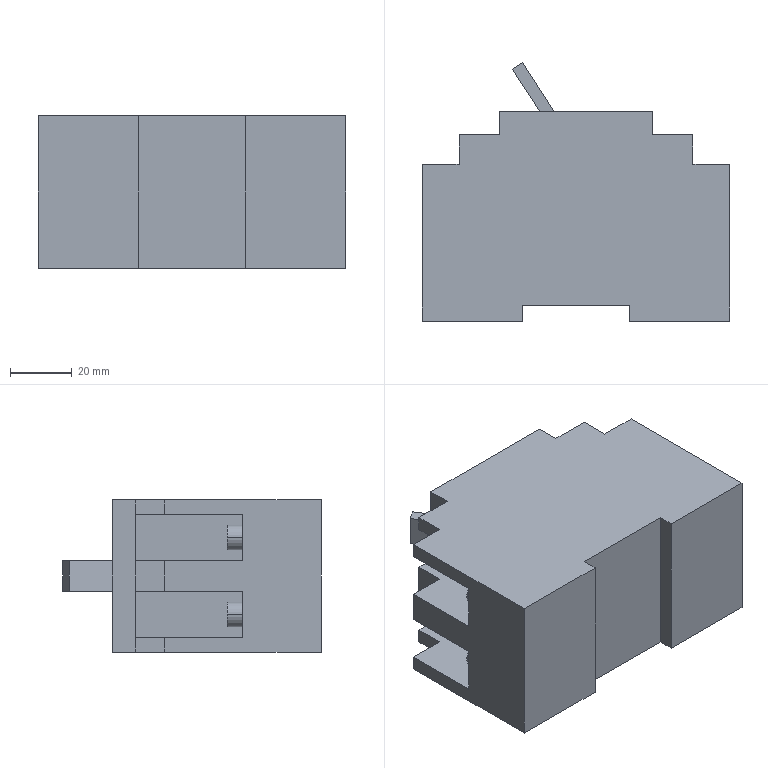Part | STEP file | Three-control-box air switch | 1 solid | 59 faces | box 100 x 84.014 x 49.5 mm | volume 273026 mm3 | plane 51 | cylinder 8 | commonest cylinder face diameters 8 x8